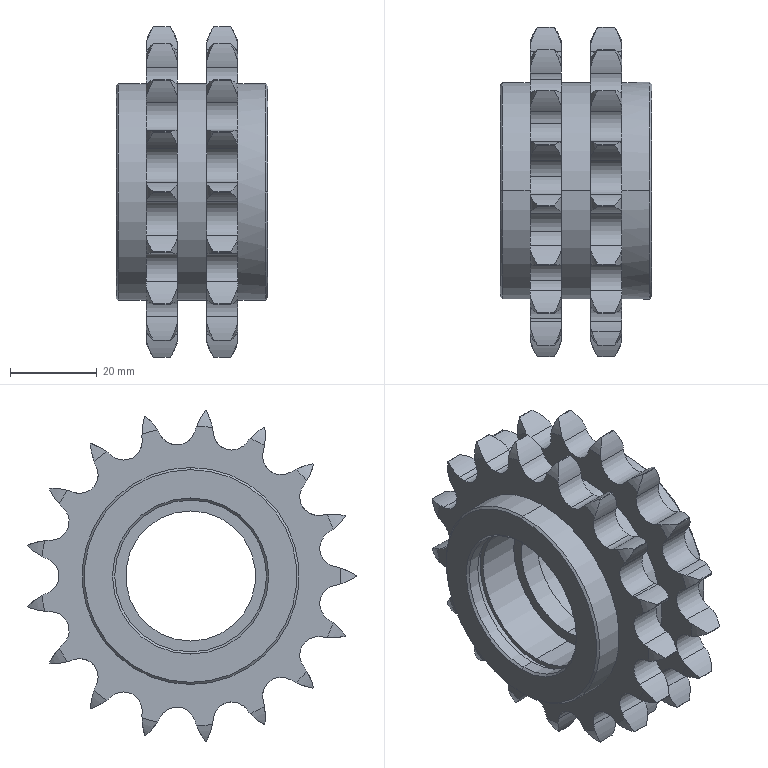Part | SolidWorks | features BaseBody 1 | 1 solid | 260 faces | box 35 x 75.844 x 76.169 mm | volume 56520 mm3 | cylinder 172 | spline 68 | plane 12 | cone 8 | commonest cylinder face diameters 30.636 x72 8.51 x46 76.481 x34 35 x8 50 x6 37 x4